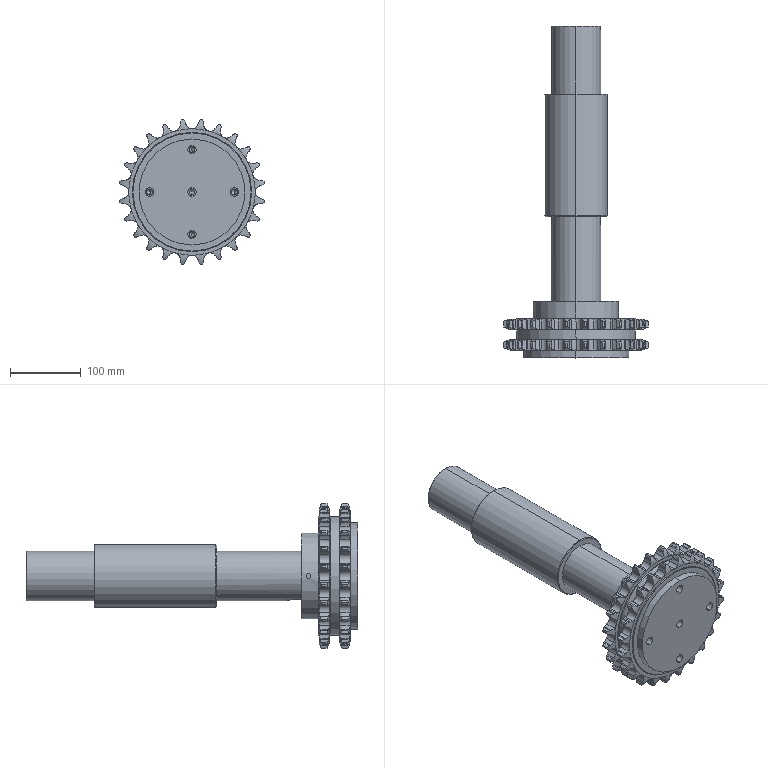Part | SolidWorks | 3 solids | 601 faces | box 204.614 x 469.5 x 204.614 mm | volume 3507608 mm3 | cylinder 356 | plane 115 | torus 104 | cone 26 | commonest cylinder face diameters 22.999 x100 41.467 x100 16.059 x62 206 x48 8.5 x12 12 x10